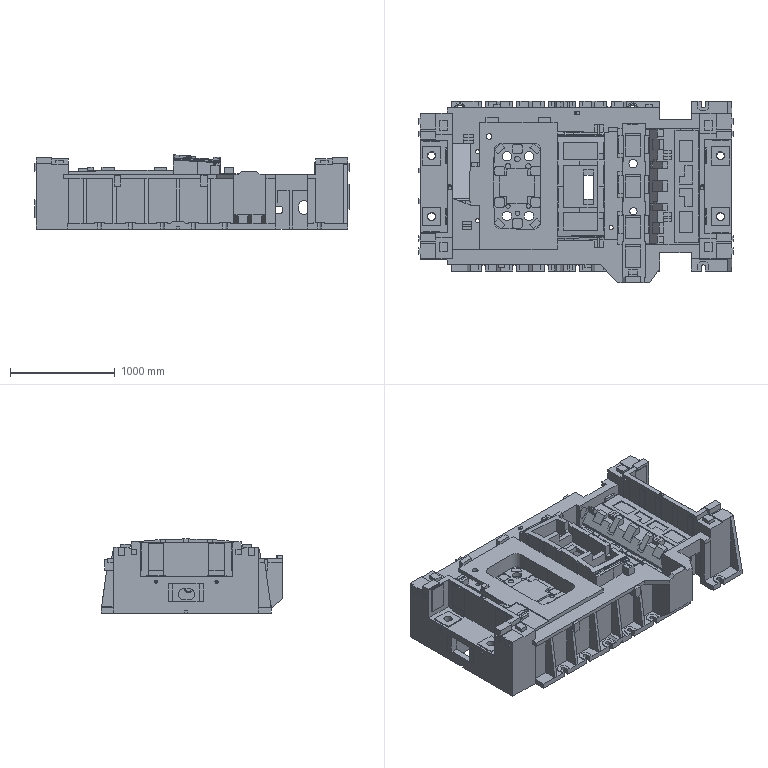Part | NX | features solid 2 | 1 solid | 1967 faces | box 3000 x 1730 x 707.86 mm | volume 883612300 mm3 | plane 1558 | cylinder 329 | spline 78 | cone 2 | commonest cylinder face diameters 80 x97 60 x56 100 x40 30 x38 10 x23 40 x22